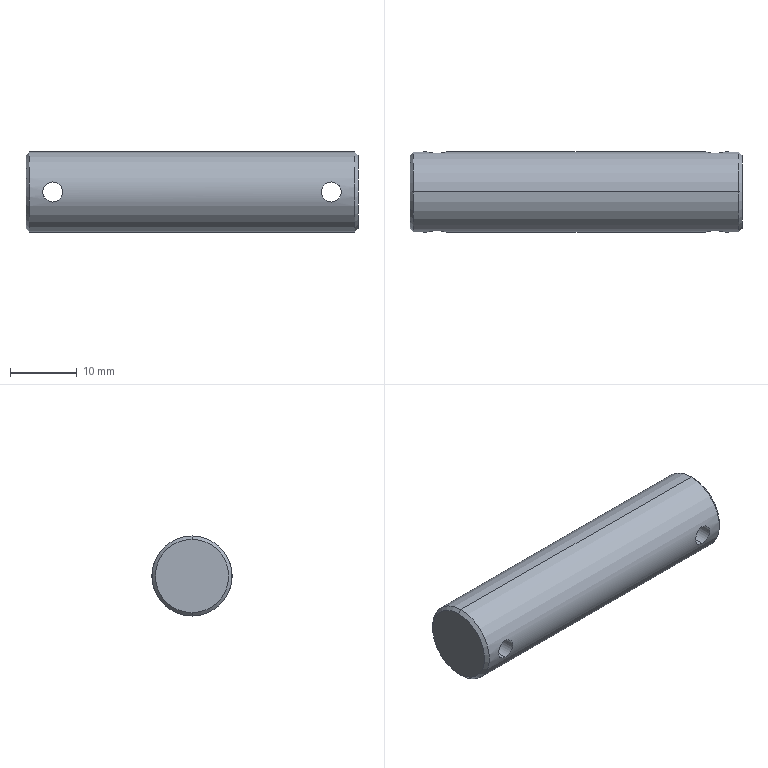Part | SolidWorks | features BaseBody 1 | 1 solid | 12 faces | box 49.7 x 12 x 12 mm | volume 5443 mm3 | cylinder 6 | cone 4 | plane 2 | commonest cylinder face diameters 3 x4 12 x2
STEP:
#1=CARTESIAN_POINT('',(-379.15,2327.809,-1291.));
#2=VERTEX_POINT('',#1);
#3=CARTESIAN_POINT('',(-379.15,2327.809,-1294.));
#4=VERTEX_POINT('',#3);
#5=CARTESIAN_POINT('',(-379.15,2327.809,-1291.));
#6=CARTESIAN_POINT('',(-379.25,2327.809,-1291.));
#7=CARTESIAN_POINT('',(-379.347,2327.812,-1291.01));
#8=CARTESIAN_POINT('',(-379.54,2327.822,-1291.048));
#9=CARTESIAN_POINT('',(-379.635,2327.829,-1291.077));
#10=CARTESIAN_POINT('',(-379.816,2327.847,-1291.153));
#11=CARTESIAN_POINT('',(-379.902,2327.857,-1291.199));
#12=CARTESIAN_POINT('',(-380.065,2327.881,-1291.307));
#13=CARTESIAN_POINT('',(-380.142,2327.893,-1291.371));
#14=CARTESIAN_POINT('',(-380.348,2327.93,-1291.577));
#15=CARTESIAN_POINT('',(-380.46,2327.955,-1291.744));
#16=CARTESIAN_POINT('',(-380.61,2327.99,-1292.104));
#17=CARTESIAN_POINT('',(-380.65,2328.,-1292.302));
#18=CARTESIAN_POINT('',(-380.65,2328.,-1292.601));
#19=CARTESIAN_POINT('',(-380.64,2327.997,-1292.698));
#20=CARTESIAN_POINT('',(-380.602,2327.988,-1292.891));
#21=CARTESIAN_POINT('',(-380.572,2327.981,-1292.986));
#22=CARTESIAN_POINT('',(-380.497,2327.963,-1293.167));
#23=CARTESIAN_POINT('',(-380.451,2327.953,-1293.253));
#24=CARTESIAN_POINT('',(-380.342,2327.93,-1293.416));
#25=CARTESIAN_POINT('',(-380.279,2327.918,-1293.493));
#26=CARTESIAN_POINT('',(-380.072,2327.881,-1293.699));
#27=CARTESIAN_POINT('',(-379.905,2327.856,-1293.811));
#28=CARTESIAN_POINT('',(-379.544,2327.82,-1293.96));
#29=CARTESIAN_POINT('',(-379.347,2327.809,-1294.));
#30=CARTESIAN_POINT('',(-379.15,2327.809,-1294.));
#31=B_SPLINE_CURVE_WITH_KNOTS('',3,(#5,#6,#7,#8,#9,#10,#11,#12,#13,#14,#15,#16,#17,#18,#19,#20,#21,#22,#23,#24,#25,#26,#27,#28,#29,#30),.UNSPECIFIED.,.F.,.F.,(4,2,2,2,2,2,2,2,2,2,2,2,4),(0.00706,0.007354,0.007648,0.007942,0.008236,0.008825,0.009413,0.009707,0.01,0.0103,0.01059,0.01118,0.01177),.UNSPECIFIED.);
#32=EDGE_CURVE('',#2,#4,#31,.T.);
#33=ORIENTED_EDGE('',*,*,#32,.T.);
#34=CARTESIAN_POINT('',(-379.15,2327.809,-1294.));
#35=CARTESIAN_POINT('',(-379.052,2327.809,-1294.));
#36=CARTESIAN_POINT('',(-378.952,2327.812,-1293.99));
#37=CARTESIAN_POINT('',(-378.759,2327.822,-1293.952));
#38=CARTESIAN_POINT('',(-378.666,2327.829,-1293.923));
#39=CARTESIAN_POINT('',(-378.393,2327.856,-1293.81));
#40=CARTESIAN_POINT('',(-378.228,2327.881,-1293.7));
#41=CARTESIAN_POINT('',(-378.02,2327.918,-1293.491));
#42=CARTESIAN_POINT('',(-377.958,2327.93,-1293.416));
#43=CARTESIAN_POINT('',(-377.85,2327.953,-1293.254));
#44=CARTESIAN_POINT('',(-377.802,2327.964,-1293.166));
#45=CARTESIAN_POINT('',(-377.69,2327.99,-1292.895));
#46=CARTESIAN_POINT('',(-377.65,2328.,-1292.699));
#47=CARTESIAN_POINT('',(-377.65,2328.,-1292.4));
#48=CARTESIAN_POINT('',(-377.66,2327.998,-1292.303));
#49=CARTESIAN_POINT('',(-377.698,2327.988,-1292.11));
#50=CARTESIAN_POINT('',(-377.727,2327.981,-1292.015));
#51=CARTESIAN_POINT('',(-377.803,2327.964,-1291.834));
#52=CARTESIAN_POINT('',(-377.849,2327.953,-1291.748));
#53=CARTESIAN_POINT('',(-377.957,2327.93,-1291.585));
#54=CARTESIAN_POINT('',(-378.02,2327.918,-1291.508));
#55=CARTESIAN_POINT('',(-378.227,2327.881,-1291.302));
#56=CARTESIAN_POINT('',(-378.393,2327.856,-1291.19));
#57=CARTESIAN_POINT('',(-378.754,2327.82,-1291.04));
#58=CARTESIAN_POINT('',(-378.951,2327.809,-1291.));
#59=CARTESIAN_POINT('',(-379.15,2327.809,-1291.));
#60=B_SPLINE_CURVE_WITH_KNOTS('',3,(#34,#35,#36,#37,#38,#39,#40,#41,#42,#43,#44,#45,#46,#47,#48,#49,#50,#51,#52,#53,#54,#55,#56,#57,#58,#59),.UNSPECIFIED.,.F.,.F.,(4,2,2,2,2,2,2,2,2,2,2,2,4),(0.002355,0.002649,0.002943,0.003531,0.003825,0.004119,0.004707,0.005001,0.005295,0.005589,0.005883,0.006471,0.00706),.UNSPECIFIED.);
#61=EDGE_CURVE('',#4,#2,#60,.T.);
#62=ORIENTED_EDGE('',*,*,#61,.T.);
#63=EDGE_LOOP('',(#33,#62));
#64=FACE_BOUND('',#63,.T.);
#65=CARTESIAN_POINT('',(-420.85,2327.809,-1291.));
#66=VERTEX_POINT('',#65);
#67=CARTESIAN_POINT('',(-420.85,2327.809,-1294.));
#68=VERTEX_POINT('',#67);
#69=CARTESIAN_POINT('',(-420.85,2327.809,-1291.));
#70=CARTESIAN_POINT('',(-420.95,2327.809,-1291.));
#71=CARTESIAN_POINT('',(-421.047,2327.812,-1291.01));
#72=CARTESIAN_POINT('',(-421.24,2327.822,-1291.048));
#73=CARTESIAN_POINT('',(-421.335,2327.829,-1291.077));
#74=CARTESIAN_POINT('',(-421.516,2327.847,-1291.153));
#75=CARTESIAN_POINT('',(-421.602,2327.857,-1291.199));
#76=CARTESIAN_POINT('',(-421.765,2327.881,-1291.307));
#77=CARTESIAN_POINT('',(-421.842,2327.893,-1291.371));
#78=CARTESIAN_POINT('',(-422.048,2327.93,-1291.577));
#79=CARTESIAN_POINT('',(-422.16,2327.955,-1291.744));
#80=CARTESIAN_POINT('',(-422.31,2327.99,-1292.104));
#81=CARTESIAN_POINT('',(-422.35,2328.,-1292.302));
#82=CARTESIAN_POINT('',(-422.35,2328.,-1292.601));
#83=CARTESIAN_POINT('',(-422.34,2327.997,-1292.698));
#84=CARTESIAN_POINT('',(-422.302,2327.988,-1292.891));
#85=CARTESIAN_POINT('',(-422.272,2327.981,-1292.986));
#86=CARTESIAN_POINT('',(-422.197,2327.963,-1293.167));
#87=CARTESIAN_POINT('',(-422.151,2327.953,-1293.253));
#88=CARTESIAN_POINT('',(-422.042,2327.93,-1293.416));
#89=CARTESIAN_POINT('',(-421.979,2327.918,-1293.493));
#90=CARTESIAN_POINT('',(-421.772,2327.881,-1293.699));
#91=CARTESIAN_POINT('',(-421.605,2327.856,-1293.811));
#92=CARTESIAN_POINT('',(-421.244,2327.82,-1293.96));
#93=CARTESIAN_POINT('',(-421.047,2327.809,-1294.));
#94=CARTESIAN_POINT('',(-420.85,2327.809,-1294.));
#95=B_SPLINE_CURVE_WITH_KNOTS('',3,(#69,#70,#71,#72,#73,#74,#75,#76,#77,#78,#79,#80,#81,#82,#83,#84,#85,#86,#87,#88,#89,#90,#91,#92,#93,#94),.UNSPECIFIED.,.F.,.F.,(4,2,2,2,2,2,2,2,2,2,2,2,4),(0.00706,0.007354,0.007648,0.007942,0.008236,0.008825,0.009413,0.009707,0.01,0.0103,0.01059,0.01118,0.01177),.UNSPECIFIED.);
#96=EDGE_CURVE('',#66,#68,#95,.T.);
#97=ORIENTED_EDGE('',*,*,#96,.T.);
#98=CARTESIAN_POINT('',(-420.85,2327.809,-1294.));
#99=CARTESIAN_POINT('',(-420.752,2327.809,-1294.));
#100=CARTESIAN_POINT('',(-420.652,2327.812,-1293.99));
#101=CARTESIAN_POINT('',(-420.459,2327.822,-1293.952));
#102=CARTESIAN_POINT('',(-420.366,2327.829,-1293.923));
#103=CARTESIAN_POINT('',(-420.093,2327.856,-1293.81));
#104=CARTESIAN_POINT('',(-419.928,2327.881,-1293.7));
#105=CARTESIAN_POINT('',(-419.72,2327.918,-1293.491));
#106=CARTESIAN_POINT('',(-419.658,2327.93,-1293.416));
#107=CARTESIAN_POINT('',(-419.55,2327.953,-1293.254));
#108=CARTESIAN_POINT('',(-419.502,2327.964,-1293.166));
#109=CARTESIAN_POINT('',(-419.39,2327.99,-1292.895));
#110=CARTESIAN_POINT('',(-419.35,2328.,-1292.699));
#111=CARTESIAN_POINT('',(-419.35,2328.,-1292.4));
#112=CARTESIAN_POINT('',(-419.36,2327.998,-1292.303));
#113=CARTESIAN_POINT('',(-419.398,2327.988,-1292.11));
#114=CARTESIAN_POINT('',(-419.427,2327.981,-1292.015));
#115=CARTESIAN_POINT('',(-419.503,2327.964,-1291.834));
#116=CARTESIAN_POINT('',(-419.549,2327.953,-1291.748));
#117=CARTESIAN_POINT('',(-419.657,2327.93,-1291.585));
#118=CARTESIAN_POINT('',(-419.72,2327.918,-1291.508));
#119=CARTESIAN_POINT('',(-419.927,2327.881,-1291.302));
#120=CARTESIAN_POINT('',(-420.093,2327.856,-1291.19));
#121=CARTESIAN_POINT('',(-420.454,2327.82,-1291.04));
#122=CARTESIAN_POINT('',(-420.651,2327.809,-1291.));
#123=CARTESIAN_POINT('',(-420.85,2327.809,-1291.));
#124=B_SPLINE_CURVE_WITH_KNOTS('',3,(#98,#99,#100,#101,#102,#103,#104,#105,#106,#107,#108,#109,#110,#111,#112,#113,#114,#115,#116,#117,#118,#119,#120,#121,#122,#123),.UNSPECIFIED.,.F.,.F.,(4,2,2,2,2,2,2,2,2,2,2,2,4),(0.002355,0.002649,0.002943,0.003531,0.003825,0.004119,0.004707,0.005001,0.005295,0.005589,0.005883,0.006471,0.00706),.UNSPECIFIED.);
#125=EDGE_CURVE('',#68,#66,#124,.T.);
#126=ORIENTED_EDGE('',*,*,#125,.T.);
#127=EDGE_LOOP('',(#97,#126));
#128=FACE_BOUND('',#127,.T.);
#129=CARTESIAN_POINT('',(-424.35,2322.,-1298.5));
#130=VERTEX_POINT('',#129);
#131=CARTESIAN_POINT('',(-424.35,2322.,-1286.5));
#132=VERTEX_POINT('',#131);
#133=CARTESIAN_POINT('',(-424.35,2322.,-1292.5));
#134=DIRECTION('',(1.,0.,0.));
#135=DIRECTION('',(0.,0.,-1.));
#136=AXIS2_PLACEMENT_3D('',#133,#134,#135);
#137=CIRCLE('',#136,6.);
#138=EDGE_CURVE('',#130,#132,#137,.T.);
#139=ORIENTED_EDGE('',*,*,#138,.T.);
#140=CARTESIAN_POINT('',(-375.65,2322.,-1286.5));
#141=VERTEX_POINT('',#140);
#142=CARTESIAN_POINT('',(-400.,2322.,-1286.5));
#143=DIRECTION('',(1.,0.,0.));
#144=VECTOR('',#143,1000.);
#145=LINE('',#142,#144);
#146=EDGE_CURVE('',#132,#141,#145,.T.);
#147=ORIENTED_EDGE('',*,*,#146,.T.);
#148=CARTESIAN_POINT('',(-375.65,2322.,-1298.5));
#149=VERTEX_POINT('',#148);
#150=CARTESIAN_POINT('',(-375.65,2322.,-1292.5));
#151=DIRECTION('',(-1.,0.,0.));
#152=DIRECTION('',(0.,0.,-1.));
#153=AXIS2_PLACEMENT_3D('',#150,#151,#152);
#154=CIRCLE('',#153,6.);
#155=EDGE_CURVE('',#141,#149,#154,.T.);
#156=ORIENTED_EDGE('',*,*,#155,.T.);
#157=CARTESIAN_POINT('',(-400.,2322.,-1298.5));
#158=DIRECTION('',(1.,0.,0.));
#159=VECTOR('',#158,1000.);
#160=LINE('',#157,#159);
#161=EDGE_CURVE('',#130,#149,#160,.T.);
#162=ORIENTED_EDGE('',*,*,#161,.F.);
#163=EDGE_LOOP('',(#139,#147,#156,#162));
#164=FACE_OUTER_BOUND('',#163,.T.);
#165=CARTESIAN_POINT('',(-400.,2322.,-1292.5));
#166=DIRECTION('',(1.,0.,0.));
#167=DIRECTION('',(0.,0.,-1.));
#168=AXIS2_PLACEMENT_3D('',#165,#166,#167);
#169=CYLINDRICAL_SURFACE('',#168,6.);
#170=ADVANCED_FACE('',(#64,#128,#164),#169,.T.);
#171=CARTESIAN_POINT('',(-424.85,2322.,-1298.));
#172=VERTEX_POINT('',#171);
#173=CARTESIAN_POINT('',(-424.85,2322.,-1287.));
#174=VERTEX_POINT('',#173);
#175=CARTESIAN_POINT('',(-424.85,2322.,-1292.5));
#176=DIRECTION('',(1.,0.,0.));
#177=DIRECTION('',(0.,0.,-1.));
#178=AXIS2_PLACEMENT_3D('',#175,#176,#177);
#179=CIRCLE('',#178,5.5);
#180=EDGE_CURVE('',#172,#174,#179,.T.);
#181=ORIENTED_EDGE('',*,*,#180,.T.);
#182=CARTESIAN_POINT('',(-424.35,2322.,-1286.5));
#183=DIRECTION('',(0.7071,0.,0.7071));
#184=VECTOR('',#183,1000.);
#185=LINE('',#182,#184);
#186=EDGE_CURVE('',#174,#132,#185,.T.);
#187=ORIENTED_EDGE('',*,*,#186,.T.);
#188=ORIENTED_EDGE('',*,*,#138,.F.);
#189=CARTESIAN_POINT('',(-424.35,2322.,-1298.5));
#190=DIRECTION('',(0.7071,0.,-0.7071));
#191=VECTOR('',#190,1000.);
#192=LINE('',#189,#191);
#193=EDGE_CURVE('',#172,#130,#192,.T.);
#194=ORIENTED_EDGE('',*,*,#193,.F.);
#195=EDGE_LOOP('',(#181,#187,#188,#194));
#196=FACE_OUTER_BOUND('',#195,.T.);
#197=CARTESIAN_POINT('',(-424.35,2322.,-1292.5));
#198=DIRECTION('',(1.,0.,0.));
#199=DIRECTION('',(0.,0.,-1.));
#200=AXIS2_PLACEMENT_3D('',#197,#198,#199);
#201=CONICAL_SURFACE('',#200,6.,0.7854);
#202=ADVANCED_FACE('',(#196),#201,.T.);
#203=CARTESIAN_POINT('',(-420.85,2316.191,-1294.));
#204=VERTEX_POINT('',#203);
#205=CARTESIAN_POINT('',(-420.85,2316.191,-1291.));
#206=VERTEX_POINT('',#205);
#207=CARTESIAN_POINT('',(-420.85,2316.191,-1294.));
#208=CARTESIAN_POINT('',(-420.948,2316.191,-1294.));
#209=CARTESIAN_POINT('',(-421.048,2316.188,-1293.99));
#210=CARTESIAN_POINT('',(-421.241,2316.178,-1293.952));
#211=CARTESIAN_POINT('',(-421.334,2316.171,-1293.923));
#212=CARTESIAN_POINT('',(-421.607,2316.144,-1293.81));
#213=CARTESIAN_POINT('',(-421.772,2316.119,-1293.7));
#214=CARTESIAN_POINT('',(-421.98,2316.082,-1293.491));
#215=CARTESIAN_POINT('',(-422.042,2316.07,-1293.416));
#216=CARTESIAN_POINT('',(-422.15,2316.047,-1293.254));
#217=CARTESIAN_POINT('',(-422.198,2316.036,-1293.166));
#218=CARTESIAN_POINT('',(-422.31,2316.01,-1292.895));
#219=CARTESIAN_POINT('',(-422.35,2316.,-1292.699));
#220=CARTESIAN_POINT('',(-422.35,2316.,-1292.4));
#221=CARTESIAN_POINT('',(-422.34,2316.002,-1292.303));
#222=CARTESIAN_POINT('',(-422.302,2316.012,-1292.11));
#223=CARTESIAN_POINT('',(-422.273,2316.019,-1292.015));
#224=CARTESIAN_POINT('',(-422.197,2316.036,-1291.834));
#225=CARTESIAN_POINT('',(-422.151,2316.047,-1291.748));
#226=CARTESIAN_POINT('',(-422.043,2316.07,-1291.585));
#227=CARTESIAN_POINT('',(-421.98,2316.082,-1291.508));
#228=CARTESIAN_POINT('',(-421.773,2316.119,-1291.302));
#229=CARTESIAN_POINT('',(-421.607,2316.144,-1291.19));
#230=CARTESIAN_POINT('',(-421.246,2316.18,-1291.04));
#231=CARTESIAN_POINT('',(-421.049,2316.191,-1291.));
#232=CARTESIAN_POINT('',(-420.85,2316.191,-1291.));
#233=B_SPLINE_CURVE_WITH_KNOTS('',3,(#207,#208,#209,#210,#211,#212,#213,#214,#215,#216,#217,#218,#219,#220,#221,#222,#223,#224,#225,#226,#227,#228,#229,#230,#231,#232),.UNSPECIFIED.,.F.,.F.,(4,2,2,2,2,2,2,2,2,2,2,2,4),(0.002355,0.002649,0.002943,0.003531,0.003825,0.004119,0.004707,0.005001,0.005295,0.005589,0.005883,0.006471,0.00706),.UNSPECIFIED.);
#234=EDGE_CURVE('',#204,#206,#233,.T.);
#235=ORIENTED_EDGE('',*,*,#234,.F.);
#236=CARTESIAN_POINT('',(-420.85,2332.,-1294.));
#237=DIRECTION('',(0.,1.,0.));
#238=VECTOR('',#237,1000.);
#239=LINE('',#236,#238);
#240=EDGE_CURVE('',#204,#68,#239,.T.);
#241=ORIENTED_EDGE('',*,*,#240,.T.);
#242=ORIENTED_EDGE('',*,*,#96,.F.);
#243=CARTESIAN_POINT('',(-420.85,2332.,-1291.));
#244=DIRECTION('',(0.,1.,0.));
#245=VECTOR('',#244,1000.);
#246=LINE('',#243,#245);
#247=EDGE_CURVE('',#206,#66,#246,.T.);
#248=ORIENTED_EDGE('',*,*,#247,.F.);
#249=EDGE_LOOP('',(#235,#241,#242,#248));
#250=FACE_OUTER_BOUND('',#249,.T.);
#251=CARTESIAN_POINT('',(-420.85,2332.,-1292.5));
#252=DIRECTION('',(0.,1.,0.));
#253=DIRECTION('',(0.,0.,1.));
#254=AXIS2_PLACEMENT_3D('',#251,#252,#253);
#255=CYLINDRICAL_SURFACE('',#254,1.5);
#256=ADVANCED_FACE('',(#250),#255,.F.);
#257=CARTESIAN_POINT('',(-379.15,2316.191,-1294.));
#258=VERTEX_POINT('',#257);
#259=CARTESIAN_POINT('',(-379.15,2316.191,-1291.));
#260=VERTEX_POINT('',#259);
#261=CARTESIAN_POINT('',(-379.15,2316.191,-1294.));
#262=CARTESIAN_POINT('',(-379.248,2316.191,-1294.));
#263=CARTESIAN_POINT('',(-379.348,2316.188,-1293.99));
#264=CARTESIAN_POINT('',(-379.541,2316.178,-1293.952));
#265=CARTESIAN_POINT('',(-379.634,2316.171,-1293.923));
#266=CARTESIAN_POINT('',(-379.907,2316.144,-1293.81));
#267=CARTESIAN_POINT('',(-380.072,2316.119,-1293.7));
#268=CARTESIAN_POINT('',(-380.28,2316.082,-1293.491));
#269=CARTESIAN_POINT('',(-380.342,2316.07,-1293.416));
#270=CARTESIAN_POINT('',(-380.45,2316.047,-1293.254));
#271=CARTESIAN_POINT('',(-380.498,2316.036,-1293.166));
#272=CARTESIAN_POINT('',(-380.61,2316.01,-1292.895));
#273=CARTESIAN_POINT('',(-380.65,2316.,-1292.699));
#274=CARTESIAN_POINT('',(-380.65,2316.,-1292.4));
#275=CARTESIAN_POINT('',(-380.64,2316.002,-1292.303));
#276=CARTESIAN_POINT('',(-380.602,2316.012,-1292.11));
#277=CARTESIAN_POINT('',(-380.573,2316.019,-1292.015));
#278=CARTESIAN_POINT('',(-380.497,2316.036,-1291.834));
#279=CARTESIAN_POINT('',(-380.451,2316.047,-1291.748));
#280=CARTESIAN_POINT('',(-380.343,2316.07,-1291.585));
#281=CARTESIAN_POINT('',(-380.28,2316.082,-1291.508));
#282=CARTESIAN_POINT('',(-380.073,2316.119,-1291.302));
#283=CARTESIAN_POINT('',(-379.907,2316.144,-1291.19));
#284=CARTESIAN_POINT('',(-379.546,2316.18,-1291.04));
#285=CARTESIAN_POINT('',(-379.349,2316.191,-1291.));
#286=CARTESIAN_POINT('',(-379.15,2316.191,-1291.));
#287=B_SPLINE_CURVE_WITH_KNOTS('',3,(#261,#262,#263,#264,#265,#266,#267,#268,#269,#270,#271,#272,#273,#274,#275,#276,#277,#278,#279,#280,#281,#282,#283,#284,#285,#286),.UNSPECIFIED.,.F.,.F.,(4,2,2,2,2,2,2,2,2,2,2,2,4),(0.002355,0.002649,0.002943,0.003531,0.003825,0.004119,0.004707,0.005001,0.005295,0.005589,0.005883,0.006471,0.00706),.UNSPECIFIED.);
#288=EDGE_CURVE('',#258,#260,#287,.T.);
#289=ORIENTED_EDGE('',*,*,#288,.F.);
#290=CARTESIAN_POINT('',(-379.15,2332.,-1294.));
#291=DIRECTION('',(0.,1.,0.));
#292=VECTOR('',#291,1000.);
#293=LINE('',#290,#292);
#294=EDGE_CURVE('',#258,#4,#293,.T.);
#295=ORIENTED_EDGE('',*,*,#294,.T.);
#296=ORIENTED_EDGE('',*,*,#32,.F.);
#297=CARTESIAN_POINT('',(-379.15,2332.,-1291.));
#298=DIRECTION('',(0.,1.,0.));
#299=VECTOR('',#298,1000.);
#300=LINE('',#297,#299);
#301=EDGE_CURVE('',#260,#2,#300,.T.);
#302=ORIENTED_EDGE('',*,*,#301,.F.);
#303=EDGE_LOOP('',(#289,#295,#296,#302));
#304=FACE_OUTER_BOUND('',#303,.T.);
#305=CARTESIAN_POINT('',(-379.15,2332.,-1292.5));
#306=DIRECTION('',(0.,1.,0.));
#307=DIRECTION('',(0.,0.,1.));
#308=AXIS2_PLACEMENT_3D('',#305,#306,#307);
#309=CYLINDRICAL_SURFACE('',#308,1.5);
#310=ADVANCED_FACE('',(#304),#309,.F.);
#311=CARTESIAN_POINT('',(-375.15,2322.,-1287.));
#312=VERTEX_POINT('',#311);
#313=CARTESIAN_POINT('',(-375.15,2322.,-1298.));
#314=VERTEX_POINT('',#313);
#315=CARTESIAN_POINT('',(-375.15,2322.,-1292.5));
#316=DIRECTION('',(-1.,0.,0.));
#317=DIRECTION('',(0.,0.,1.));
#318=AXIS2_PLACEMENT_3D('',#315,#316,#317);
#319=CIRCLE('',#318,5.5);
#320=EDGE_CURVE('',#312,#314,#319,.T.);
#321=ORIENTED_EDGE('',*,*,#320,.T.);
#322=CARTESIAN_POINT('',(-375.65,2322.,-1298.5));
#323=DIRECTION('',(-0.7071,0.,-0.7071));
#324=VECTOR('',#323,1000.);
#325=LINE('',#322,#324);
#326=EDGE_CURVE('',#314,#149,#325,.T.);
#327=ORIENTED_EDGE('',*,*,#326,.T.);
#328=ORIENTED_EDGE('',*,*,#155,.F.);
#329=CARTESIAN_POINT('',(-375.65,2322.,-1286.5));
#330=DIRECTION('',(-0.7071,0.,0.7071));
#331=VECTOR('',#330,1000.);
#332=LINE('',#329,#331);
#333=EDGE_CURVE('',#312,#141,#332,.T.);
#334=ORIENTED_EDGE('',*,*,#333,.F.);
#335=EDGE_LOOP('',(#321,#327,#328,#334));
#336=FACE_OUTER_BOUND('',#335,.T.);
#337=CARTESIAN_POINT('',(-375.65,2322.,-1292.5));
#338=DIRECTION('',(-1.,0.,0.));
#339=DIRECTION('',(0.,0.,1.));
#340=AXIS2_PLACEMENT_3D('',#337,#338,#339);
#341=CONICAL_SURFACE('',#340,6.,0.7854);
#342=ADVANCED_FACE('',(#336),#341,.T.);
#343=ORIENTED_EDGE('',*,*,#146,.F.);
#344=CARTESIAN_POINT('',(-424.35,2322.,-1292.5));
#345=DIRECTION('',(1.,0.,0.));
#346=DIRECTION('',(0.,0.,-1.));
#347=AXIS2_PLACEMENT_3D('',#344,#345,#346);
#348=CIRCLE('',#347,6.);
#349=EDGE_CURVE('',#132,#130,#348,.T.);
#350=ORIENTED_EDGE('',*,*,#349,.T.);
#351=ORIENTED_EDGE('',*,*,#161,.T.);
#352=CARTESIAN_POINT('',(-375.65,2322.,-1292.5));
#353=DIRECTION('',(-1.,0.,0.));
#354=DIRECTION('',(0.,0.,-1.));
#355=AXIS2_PLACEMENT_3D('',#352,#353,#354);
#356=CIRCLE('',#355,6.);
#357=EDGE_CURVE('',#149,#141,#356,.T.);
#358=ORIENTED_EDGE('',*,*,#357,.T.);
#359=EDGE_LOOP('',(#343,#350,#351,#358));
#360=FACE_OUTER_BOUND('',#359,.T.);
#361=CARTESIAN_POINT('',(-379.15,2316.191,-1291.));
#362=CARTESIAN_POINT('',(-379.05,2316.191,-1291.));
#363=CARTESIAN_POINT('',(-378.953,2316.188,-1291.01));
#364=CARTESIAN_POINT('',(-378.76,2316.178,-1291.048));
#365=CARTESIAN_POINT('',(-378.665,2316.171,-1291.077));
#366=CARTESIAN_POINT('',(-378.484,2316.153,-1291.153));
#367=CARTESIAN_POINT('',(-378.398,2316.143,-1291.199));
#368=CARTESIAN_POINT('',(-378.235,2316.119,-1291.307));
#369=CARTESIAN_POINT('',(-378.158,2316.107,-1291.371));
#370=CARTESIAN_POINT('',(-377.952,2316.07,-1291.577));
#371=CARTESIAN_POINT('',(-377.84,2316.045,-1291.744));
#372=CARTESIAN_POINT('',(-377.69,2316.01,-1292.104));
#373=CARTESIAN_POINT('',(-377.65,2316.,-1292.302));
#374=CARTESIAN_POINT('',(-377.65,2316.,-1292.601));
#375=CARTESIAN_POINT('',(-377.66,2316.003,-1292.698));
#376=CARTESIAN_POINT('',(-377.698,2316.012,-1292.891));
#377=CARTESIAN_POINT('',(-377.728,2316.019,-1292.986));
#378=CARTESIAN_POINT('',(-377.803,2316.037,-1293.167));
#379=CARTESIAN_POINT('',(-377.849,2316.047,-1293.253));
#380=CARTESIAN_POINT('',(-377.958,2316.07,-1293.416));
#381=CARTESIAN_POINT('',(-378.021,2316.082,-1293.493));
#382=CARTESIAN_POINT('',(-378.228,2316.119,-1293.699));
#383=CARTESIAN_POINT('',(-378.395,2316.144,-1293.811));
#384=CARTESIAN_POINT('',(-378.756,2316.18,-1293.96));
#385=CARTESIAN_POINT('',(-378.953,2316.191,-1294.));
#386=CARTESIAN_POINT('',(-379.15,2316.191,-1294.));
#387=B_SPLINE_CURVE_WITH_KNOTS('',3,(#361,#362,#363,#364,#365,#366,#367,#368,#369,#370,#371,#372,#373,#374,#375,#376,#377,#378,#379,#380,#381,#382,#383,#384,#385,#386),.UNSPECIFIED.,.F.,.F.,(4,2,2,2,2,2,2,2,2,2,2,2,4),(0.00706,0.007354,0.007648,0.007942,0.008236,0.008825,0.009413,0.009707,0.01,0.0103,0.01059,0.01118,0.01177),.UNSPECIFIED.);
#388=EDGE_CURVE('',#260,#258,#387,.T.);
#389=ORIENTED_EDGE('',*,*,#388,.T.);
#390=ORIENTED_EDGE('',*,*,#288,.T.);
#391=EDGE_LOOP('',(#389,#390));
#392=FACE_BOUND('',#391,.T.);
#393=CARTESIAN_POINT('',(-420.85,2316.191,-1291.));
#394=CARTESIAN_POINT('',(-420.75,2316.191,-1291.));
#395=CARTESIAN_POINT('',(-420.653,2316.188,-1291.01));
#396=CARTESIAN_POINT('',(-420.46,2316.178,-1291.048));
#397=CARTESIAN_POINT('',(-420.365,2316.171,-1291.077));
#398=CARTESIAN_POINT('',(-420.184,2316.153,-1291.153));
#399=CARTESIAN_POINT('',(-420.098,2316.143,-1291.199));
#400=CARTESIAN_POINT('',(-419.935,2316.119,-1291.307));
#401=CARTESIAN_POINT('',(-419.858,2316.107,-1291.371));
#402=CARTESIAN_POINT('',(-419.652,2316.07,-1291.577));
#403=CARTESIAN_POINT('',(-419.54,2316.045,-1291.744));
#404=CARTESIAN_POINT('',(-419.39,2316.01,-1292.104));
#405=CARTESIAN_POINT('',(-419.35,2316.,-1292.302));
#406=CARTESIAN_POINT('',(-419.35,2316.,-1292.601));
#407=CARTESIAN_POINT('',(-419.36,2316.003,-1292.698));
#408=CARTESIAN_POINT('',(-419.398,2316.012,-1292.891));
#409=CARTESIAN_POINT('',(-419.428,2316.019,-1292.986));
#410=CARTESIAN_POINT('',(-419.503,2316.037,-1293.167));
#411=CARTESIAN_POINT('',(-419.549,2316.047,-1293.253));
#412=CARTESIAN_POINT('',(-419.658,2316.07,-1293.416));
#413=CARTESIAN_POINT('',(-419.721,2316.082,-1293.493));
#414=CARTESIAN_POINT('',(-419.928,2316.119,-1293.699));
#415=CARTESIAN_POINT('',(-420.095,2316.144,-1293.811));
#416=CARTESIAN_POINT('',(-420.456,2316.18,-1293.96));
#417=CARTESIAN_POINT('',(-420.653,2316.191,-1294.));
#418=CARTESIAN_POINT('',(-420.85,2316.191,-1294.));
#419=B_SPLINE_CURVE_WITH_KNOTS('',3,(#393,#394,#395,#396,#397,#398,#399,#400,#401,#402,#403,#404,#405,#406,#407,#408,#409,#410,#411,#412,#413,#414,#415,#416,#417,#418),.UNSPECIFIED.,.F.,.F.,(4,2,2,2,2,2,2,2,2,2,2,2,4),(0.00706,0.007354,0.007648,0.007942,0.008236,0.008825,0.009413,0.009707,0.01,0.0103,0.01059,0.01118,0.01177),.UNSPECIFIED.);
#420=EDGE_CURVE('',#206,#204,#419,.T.);
#421=ORIENTED_EDGE('',*,*,#420,.T.);
#422=ORIENTED_EDGE('',*,*,#234,.T.);
#423=EDGE_LOOP('',(#421,#422));
#424=FACE_BOUND('',#423,.T.);
#425=CARTESIAN_POINT('',(-400.,2322.,-1292.5));
#426=DIRECTION('',(1.,0.,0.));
#427=DIRECTION('',(0.,0.,-1.));
#428=AXIS2_PLACEMENT_3D('',#425,#426,#427);
#429=CYLINDRICAL_SURFACE('',#428,6.);
#430=ADVANCED_FACE('',(#360,#392,#424),#429,.T.);
#431=ORIENTED_EDGE('',*,*,#186,.F.);
#432=CARTESIAN_POINT('',(-424.85,2322.,-1292.5));
#433=DIRECTION('',(1.,0.,0.));
#434=DIRECTION('',(0.,0.,-1.));
#435=AXIS2_PLACEMENT_3D('',#432,#433,#434);
#436=CIRCLE('',#435,5.5);
#437=EDGE_CURVE('',#174,#172,#436,.T.);
#438=ORIENTED_EDGE('',*,*,#437,.T.);
#439=ORIENTED_EDGE('',*,*,#193,.T.);
#440=ORIENTED_EDGE('',*,*,#349,.F.);
#441=EDGE_LOOP('',(#431,#438,#439,#440));
#442=FACE_OUTER_BOUND('',#441,.T.);
#443=CARTESIAN_POINT('',(-424.35,2322.,-1292.5));
#444=DIRECTION('',(1.,0.,0.));
#445=DIRECTION('',(0.,0.,-1.));
#446=AXIS2_PLACEMENT_3D('',#443,#444,#445);
#447=CONICAL_SURFACE('',#446,6.,0.7854);
#448=ADVANCED_FACE('',(#442),#447,.T.);
#449=ORIENTED_EDGE('',*,*,#240,.F.);
#450=ORIENTED_EDGE('',*,*,#420,.F.);
#451=ORIENTED_EDGE('',*,*,#247,.T.);
#452=ORIENTED_EDGE('',*,*,#125,.F.);
#453=EDGE_LOOP('',(#449,#450,#451,#452));
#454=FACE_OUTER_BOUND('',#453,.T.);
#455=CARTESIAN_POINT('',(-420.85,2332.,-1292.5));
#456=DIRECTION('',(0.,1.,0.));
#457=DIRECTION('',(0.,0.,1.));
#458=AXIS2_PLACEMENT_3D('',#455,#456,#457);
#459=CYLINDRICAL_SURFACE('',#458,1.5);
#460=ADVANCED_FACE('',(#454),#459,.F.);
#461=ORIENTED_EDGE('',*,*,#294,.F.);
#462=ORIENTED_EDGE('',*,*,#388,.F.);
#463=ORIENTED_EDGE('',*,*,#301,.T.);
#464=ORIENTED_EDGE('',*,*,#61,.F.);
#465=EDGE_LOOP('',(#461,#462,#463,#464));
#466=FACE_OUTER_BOUND('',#465,.T.);
#467=CARTESIAN_POINT('',(-379.15,2332.,-1292.5));
#468=DIRECTION('',(0.,1.,0.));
#469=DIRECTION('',(0.,0.,1.));
#470=AXIS2_PLACEMENT_3D('',#467,#468,#469);
#471=CYLINDRICAL_SURFACE('',#470,1.5);
#472=ADVANCED_FACE('',(#466),#471,.F.);
#473=ORIENTED_EDGE('',*,*,#326,.F.);
#474=CARTESIAN_POINT('',(-375.15,2322.,-1292.5));
#475=DIRECTION('',(-1.,0.,0.));
#476=DIRECTION('',(0.,0.,1.));
#477=AXIS2_PLACEMENT_3D('',#474,#475,#476);
#478=CIRCLE('',#477,5.5);
#479=EDGE_CURVE('',#314,#312,#478,.T.);
#480=ORIENTED_EDGE('',*,*,#479,.T.);
#481=ORIENTED_EDGE('',*,*,#333,.T.);
#482=ORIENTED_EDGE('',*,*,#357,.F.);
#483=EDGE_LOOP('',(#473,#480,#481,#482));
#484=FACE_OUTER_BOUND('',#483,.T.);
#485=CARTESIAN_POINT('',(-375.65,2322.,-1292.5));
#486=DIRECTION('',(-1.,0.,0.));
#487=DIRECTION('',(0.,0.,1.));
#488=AXIS2_PLACEMENT_3D('',#485,#486,#487);
#489=CONICAL_SURFACE('',#488,6.,0.7854);
#490=ADVANCED_FACE('',(#484),#489,.T.);
#491=ORIENTED_EDGE('',*,*,#180,.F.);
#492=ORIENTED_EDGE('',*,*,#437,.F.);
#493=EDGE_LOOP('',(#491,#492));
#494=FACE_OUTER_BOUND('',#493,.T.);
#495=CARTESIAN_POINT('',(-424.85,2322.,-1295.25));
#496=DIRECTION('',(-1.,0.,0.));
#497=DIRECTION('',(0.,0.,1.));
#498=AXIS2_PLACEMENT_3D('',#495,#496,#497);
#499=PLANE('',#498);
#500=ADVANCED_FACE('',(#494),#499,.T.);
#501=ORIENTED_EDGE('',*,*,#320,.F.);
#502=ORIENTED_EDGE('',*,*,#479,.F.);
#503=EDGE_LOOP('',(#501,#502));
#504=FACE_OUTER_BOUND('',#503,.T.);
#505=CARTESIAN_POINT('',(-375.15,2322.,-1295.25));
#506=DIRECTION('',(1.,0.,0.));
#507=DIRECTION('',(0.,0.,-1.));
#508=AXIS2_PLACEMENT_3D('',#505,#506,#507);
#509=PLANE('',#508);
#510=ADVANCED_FACE('',(#504),#509,.T.);
#511=CLOSED_SHELL('',(#170,#202,#256,#310,#342,#430,#448,#460,#472,#490,#500,#510));
#512=MANIFOLD_SOLID_BREP('',#511);
#513=CARTESIAN_POINT('',(0.,0.,0.));
#514=DIRECTION('',(0.,0.,1.));
#515=DIRECTION('',(1.,0.,0.));
#516=AXIS2_PLACEMENT_3D('',#513,#514,#515);
#517=(LENGTH_UNIT()NAMED_UNIT(*)SI_UNIT(.MILLI.,.METRE.));
#518=UNCERTAINTY_MEASURE_WITH_UNIT(LENGTH_MEASURE(0.00001),#517,'','');
#519=(NAMED_UNIT(*)PLANE_ANGLE_UNIT()SI_UNIT($,.RADIAN.));
#520=(NAMED_UNIT(*)SI_UNIT($,.STERADIAN.)SOLID_ANGLE_UNIT());
#521=(GEOMETRIC_REPRESENTATION_CONTEXT(3)GLOBAL_UNCERTAINTY_ASSIGNED_CONTEXT((#518))GLOBAL_UNIT_ASSIGNED_CONTEXT((#517,#519,#520))REPRESENTATION_CONTEXT('',''));
#522=ADVANCED_BREP_SHAPE_REPRESENTATION('',(#512,#516),#521);